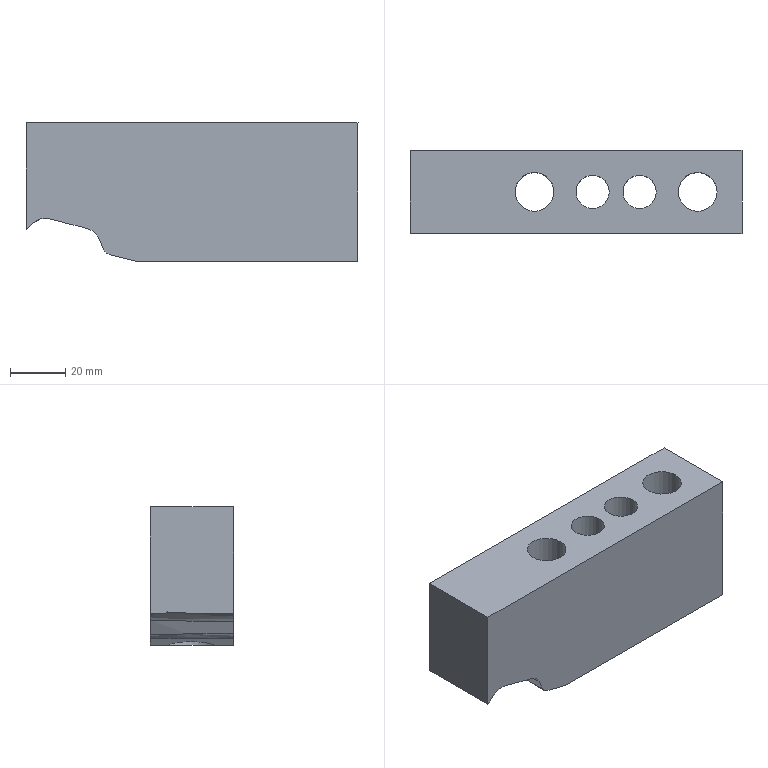Part | NX | features solid 2 | 1 solid | 23 faces | box 120 x 30 x 50 mm | volume 135438 mm3 | spline 9 | plane 8 | cylinder 6 | commonest cylinder face diameters 12 x2 14 x2 20 x2